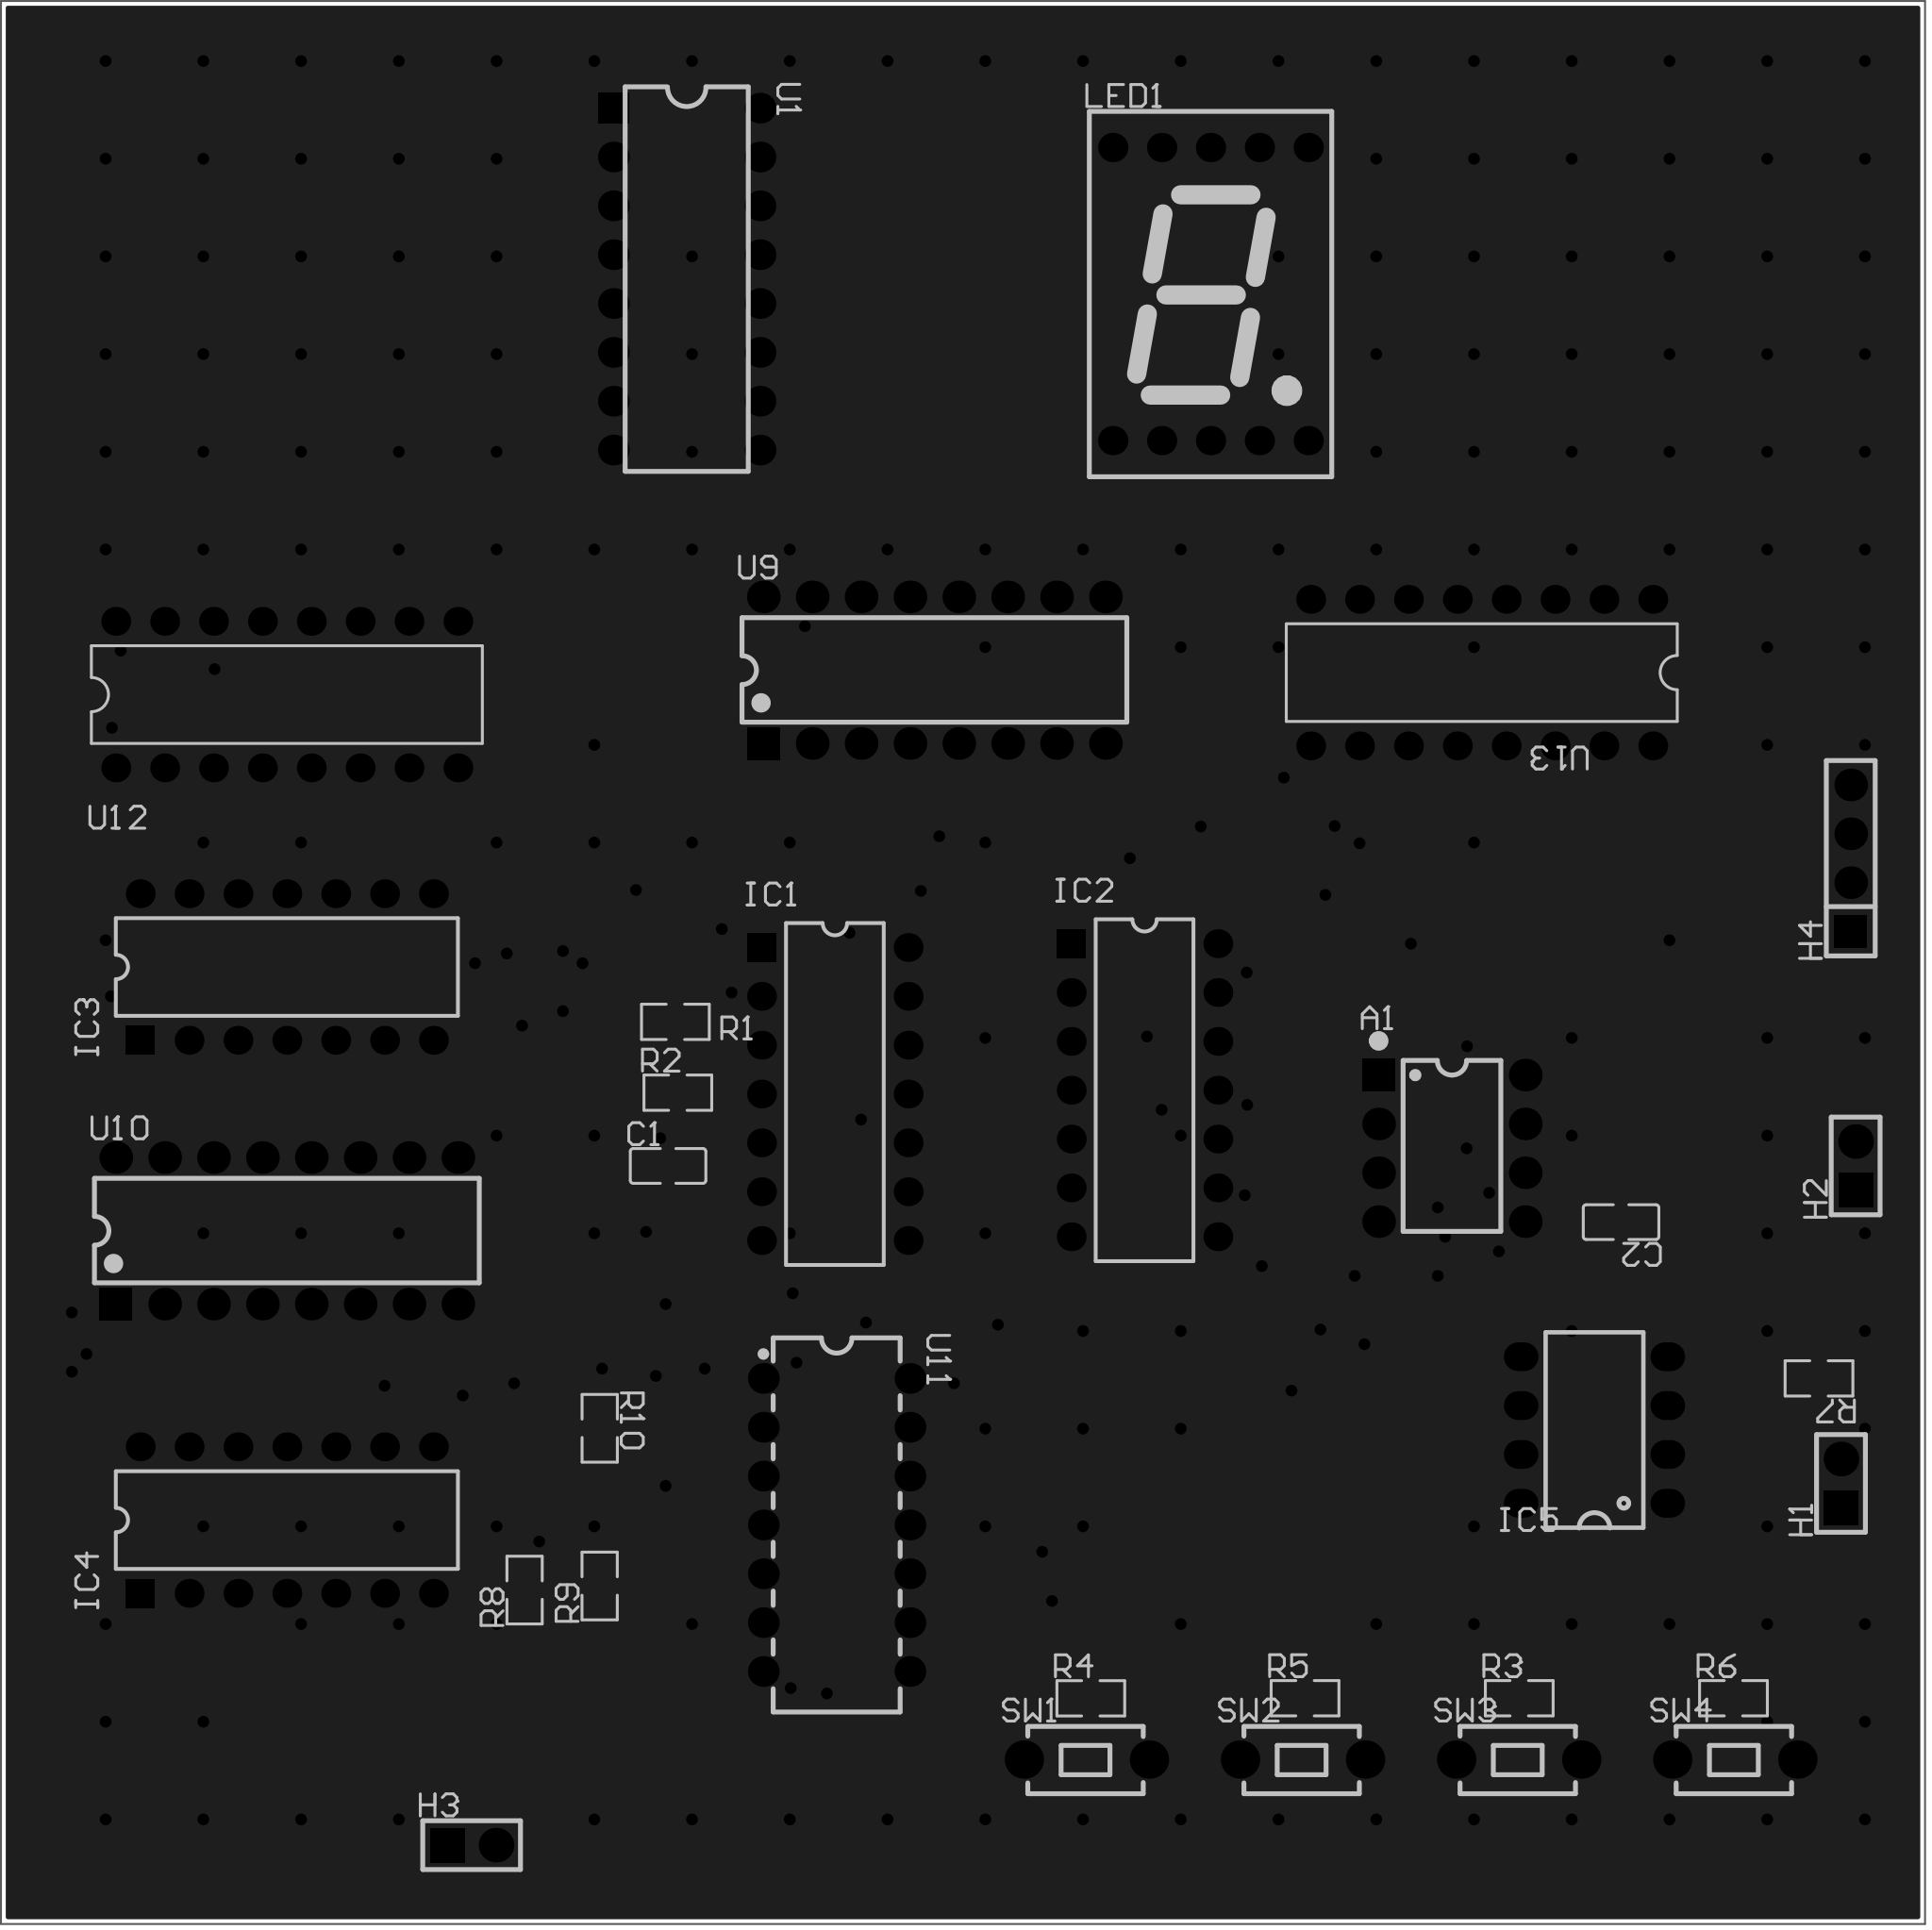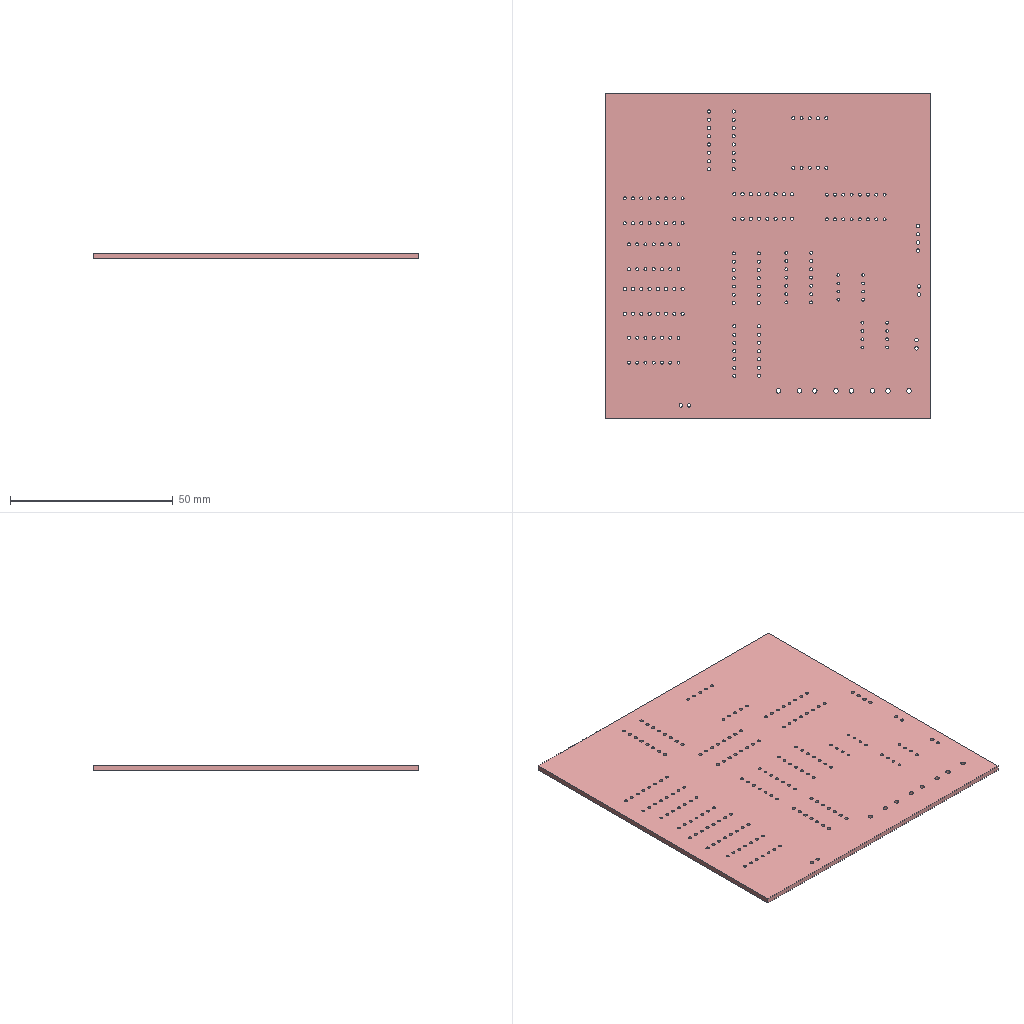Circuit board layout | Altium Designer | box 100 x 100 x 1.6 mm
Layer stack:
# Altium Designer layer stack of  (unit mm; dielectric type: 0 none, 1 core, 2 prepreg, 3 surface material)
index,name,kind,layer,copper_thickness_mm,dielectric_type,dielectric_thickness_mm,dielectric_material,dielectric_constant
0,Top Paste Mask Layer,other,,,,,,
1,Top Silkscreen Layer,other,,,,,,
2,Top Solder Mask Layer,dielectric,,,3,0.01,,3.3
3,Top Layer,copper,Top Layer,0.035,,,,
4,Dielectric1,dielectric,,,3,1.51,FR4,4.5
5,Bottom Layer,copper,Bottom Layer,0.035,,,,
6,Bottom Solder Mask Layer,dielectric,,,3,0.01,,3.3
7,Bottom Silkscreen Layer,other,,,,,,
8,Bottom Paste Mask Layer,other,,,,,,
# drill layer pairs: low layer,high layer
drill_pair,Top Layer,Bottom Layer
Part placement:
Designator,Comment,Layer,Footprint,Center-X(mm),Center-Y(mm),Rotation
A1,555_VIRTUAL,TopLayer,555-VIRTUAL,166.599,132.994,0
C1,10uF,TopLayer,C0805,125.857,132.08,0
C2,10nF,TopLayer,C0805,175.387,129.159,180
H1,,TopLayer,HDR-TH_2P-P2.54-V-M-1,186.817,115.57,90
H2,,TopLayer,HDR-TH_2P-P2.54-V-M-1,187.579,132.08,90
H3,,TopLayer,HDR-TH_2P-P2.54-V-M-1,115.647,96.76,0
H4,,TopLayer,HDR-TH_4P-P2.54-V-M,187.325,148.082,90
IC1,74LS00N,TopLayer,DIP14-300_MH,134.526,135.82,0
IC2,74LS00N,TopLayer,DIP14-300_MH,150.622,136.017,0
IC3,74LS00N,TopLayer,DIP14-300_MH,106.045,142.425,90
IC4,74LS00N,TopLayer,DIP14-300_MH,106.045,113.665,90
IC5,UA741CP,TopLayer,DIP8,174.006,118.348,90
LED1,,TopLayer,LED-SEG-TH_10P-L12.6-W19.0-P2.54-S15.24-BL,154.051,177.419,0
R1,100K,TopLayer,R0805,126.238,139.573,180
R2,20K,TopLayer,R0805,126.365,135.89,0
R3,10K,TopLayer,R0805,170.095,104.399,0
R4,10K,TopLayer,R0805,147.828,104.394,0
R5,10K,TopLayer,R0805,158.962,104.399,0
R6,10K,TopLayer,R0805,181.229,104.399,0
R7,10K,TopLayer,R0805,185.674,121.031,180
R8,30K,TopLayer,R0805,118.399,110.022,90
R9,20K,TopLayer,R0805,122.301,110.236,90
R10,10K,TopLayer,R0805,122.304,118.436,270
SW1,,TopLayer,Key_TH_3.5x6x4.3,147.603,101.212,0
SW2,,TopLayer,Key_TH_3.5x6x4.3,158.835,101.212,0
SW3,,TopLayer,Key_TH_3.5x6x4.3,170.068,101.212,0
SW4,,TopLayer,Key_TH_3.5x6x4.3,181.3,101.212,0
U1,,TopLayer,DIP-16_L19.8-W6.5-P2.54-LS7.6-BL,126.826,178.197,270
U9,,TopLayer,PDIP-16_L19.7-W6.6-P2.54-LS7.6-BL,139.7,157.861,0
U10,,TopLayer,PDIP-16_L19.7-W6.6-P2.54-LS7.6-BL,106.045,128.705,0
U11,,TopLayer,PDIP-14_L19.3-W6.4-P2.54-LS7.9-BL,134.62,113.411,270
U12,74LS138N,TopLayer,DIP-16_L20.32-W6.4-P2.54-LS7.6-BL,106.045,156.591,0
U13,74LS161DC,TopLayer,DIP-16_L20.32-W6.4-P2.54-LS7.6-BL,168.148,157.734,180
Pad and via stacks:
# Altium Designer via and pad stacks of  (unit mm). Each distinct definition once, with the count of objects using it.
# via: kind,start_layer,end_layer,hole_mm,diameter_mm,mode(0 simple;1 top-mid-bottom;2 full stack),diameter_per_layer,count,example_net
# pad: kind,layer,hole_mm,hole_type(0 round;1 square;2 slot),plating,top_size,top_shape(1 round;2 rect;3 octagon;9 rounded rect),mid_size,bottom_size,mode,footprint,size_per_layer,count,example
pad,Multi-Layer,0.8,0,plated,1.7x1.7,2,1.7x1.7,1.7x1.7,0,555-VIRTUAL,,1,A1.1
pad,Multi-Layer,0.8,0,plated,1.7x1.7,1,1.7x1.7,1.7x1.7,0,555-VIRTUAL,,7,A1.2
pad,Multi-Layer,1.1,0,plated,1.8x1.8,1,1.8x1.8,1.8x1.8,0,HDR-TH_2P-P2.54-V-M-1,,3,H1.2
pad,Multi-Layer,1.1,0,plated,1.8x1.8,2,1.8x1.8,1.8x1.8,0,HDR-TH_2P-P2.54-V-M-1,,3,H1.1
pad,Multi-Layer,1.1,0,plated,1.7x1.7,2,1.7x1.7,1.7x1.7,0,HDR-TH_4P-P2.54-V-M,,1,H4.1
pad,Multi-Layer,1.1,0,plated,1.7x1.7,1,1.7x1.7,1.7x1.7,0,HDR-TH_4P-P2.54-V-M,,3,H4.2
pad,Multi-Layer,0.9,2,plated,1.5x1.5,1,1.5x1.5,1.5x1.5,0,DIP14-300_MH,,52,IC1.8
pad,Multi-Layer,0.9,2,plated,1.5x1.5,2,1.5x1.5,1.5x1.5,0,DIP14-300_MH,,4,IC1.1
pad,Multi-Layer,0.85,0,plated,1.5x1.8,1,1.5x1.8,1.5x1.8,0,DIP8,,8,IC5.1
pad,Multi-Layer,0.9144,0,plated,1.524x1.524,1,1.524x1.524,1.524x1.524,0,LED-SEG-TH_10P-L12.6-W19.0-P2.54-S15.24-BL,,10,LED1.1
pad,Multi-Layer,1.399,0,plated,1.999x1.999,1,1.999x1.999,1.999x1.999,0,Key_TH_3.5x6x4.3,,8,SW1.A
pad,Multi-Layer,1,0,plated,1.6x1.6,1,1.6x1.6,1.6x1.6,0,DIP-16_L19.8-W6.5-P2.54-LS7.6-BL,,15,U1.16
pad,Multi-Layer,1,0,plated,1.6x1.6,2,1.6x1.6,1.6x1.6,0,DIP-16_L19.8-W6.5-P2.54-LS7.6-BL,,1,U1.1
pad,Multi-Layer,1,0,plated,1.7x1.7,2,1.7x1.7,1.7x1.7,0,PDIP-16_L19.7-W6.6-P2.54-LS7.6-BL,,2,U9.1
pad,Multi-Layer,1,0,plated,1.7x1.7,1,1.7x1.7,1.7x1.7,0,PDIP-16_L19.7-W6.6-P2.54-LS7.6-BL,,30,U9.2
pad,Multi-Layer,1,0,plated,1.6x1.6,1,1.6x1.6,1.6x1.6,0,PDIP-14_L19.3-W6.4-P2.54-LS7.9-BL,,14,U11.9
pad,Multi-Layer,0.9,0,plated,1.5x1.5,1,1.5x1.5,1.5x1.5,0,DIP-16_L20.32-W6.4-P2.54-LS7.6-BL,,32,U12.1
pad,Top Layer,0,0,plated,1.41x1.35,2,1.41x1.35,1.41x1.35,0,C0805,,4,C1.2
pad,Top Layer,0,0,plated,1.133x1.377,2,1.133x1.377,1.133x1.377,0,R0805,,20,R1.2
via,Top Layer,Bottom Layer,0.3048,0.61,0,,240,$1N72
Copper pours:
name,layer,net,type(0 solid;1 hatched;2 none)
Top Layer-GND,Top Layer,GND,0
Bottom Layer-GND,Bottom Layer,GND,0
Design rules, without the lines most boards share:
# Altium Designer design rules of  (exported by Altium Designer, unit mm)
# columns: name | kind | enabled | priority | scope1 | scope2 | descriptor | typed fields (field=value)
creepage | 65 | enabled | 1 | All | All | Creepage Distance Constraint =(0mil) (All),(All) |
copperThickness1oz_2 | 2 | enabled | 2 | All | All | Width Constraint (Min=30mil) (Max=100mil) (Preferred=30mil) (All) |